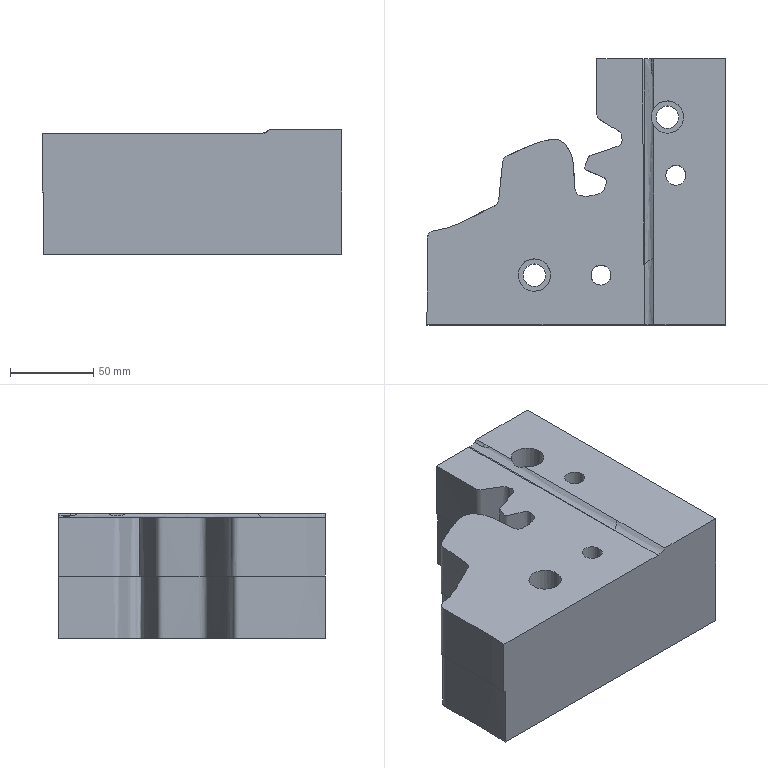Part | NX | features solid 2 | 1 solid | 22 faces | box 179.985 x 160 x 75 mm | volume 1451097 mm3 | spline 9 | plane 7 | cylinder 6 | commonest cylinder face diameters 12 x2 13.5 x2 19.5 x2